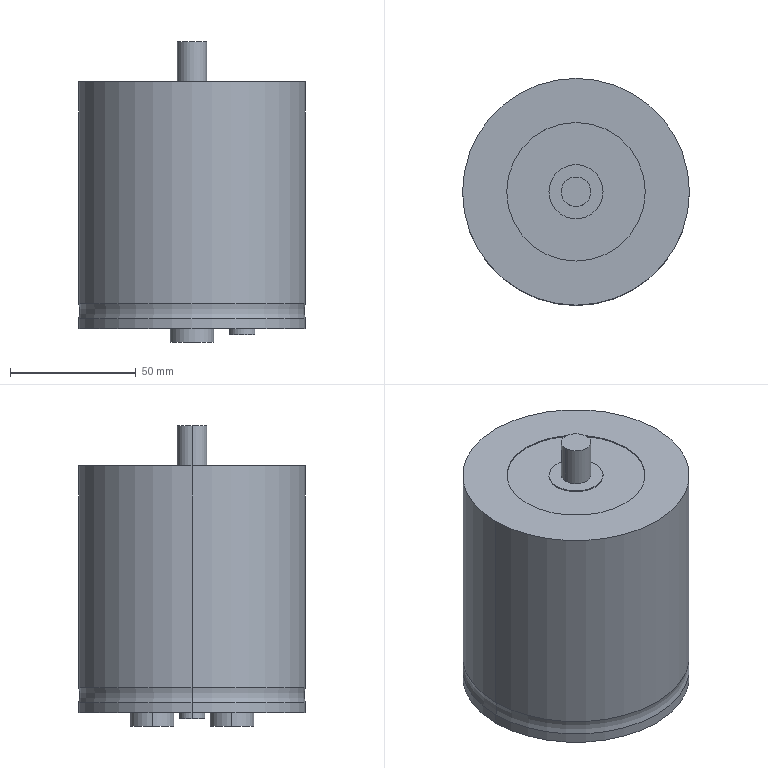Part | STEP file | 90X105 | 1 solid | 35 faces | box 90 x 90 x 119.4 mm | volume 624644 mm3 | cylinder 22 | plane 11 | torus 2 | commonest cylinder face diameters 6 x4 17.4 x4 55 x4 90 x4 10 x2 11.7 x2